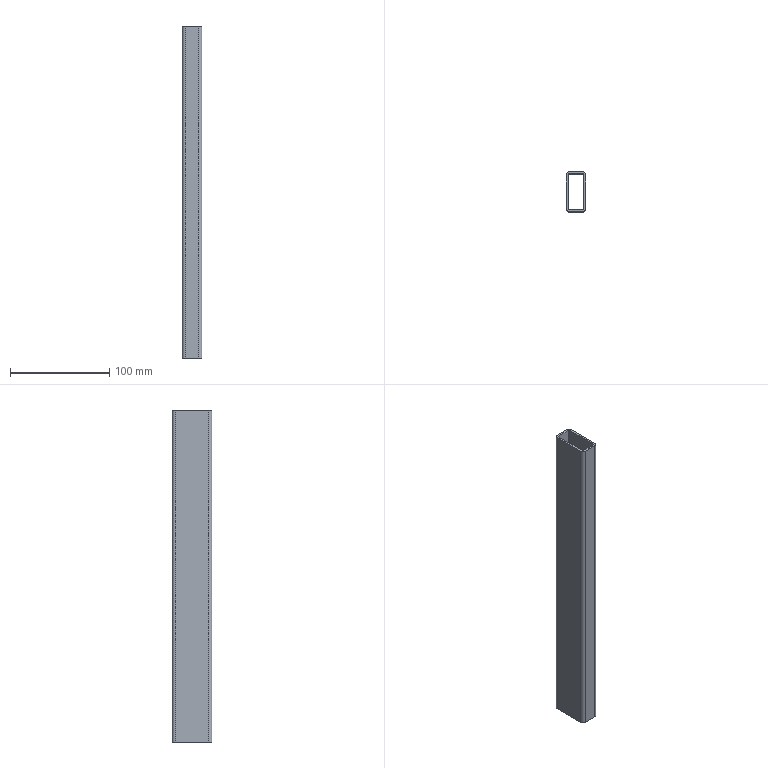Part | STEP file | CSN EN 10305-5 - 40 x 20 x 2  - 330 | 1 solid | 18 faces | box 20 x 40 x 335 mm | volume 72739 mm3 | plane 10 | cylinder 8 | commonest cylinder face diameters 2 x4 6 x4
STEP:
#1=CARTESIAN_POINT('',(0.,0.,0.));
#2=DIRECTION('',(0.,0.,1.));
#3=DIRECTION('',(1.,0.,0.));
#4=AXIS2_PLACEMENT_3D('',#1,#2,#3);
#5=CARTESIAN_POINT('',(-7.,-18.,335.));
#6=VERTEX_POINT('',#5);
#7=CARTESIAN_POINT('',(7.,-18.,335.));
#8=VERTEX_POINT('',#7);
#9=CARTESIAN_POINT('',(3.5,-18.,335.));
#10=DIRECTION('',(1.,0.,0.));
#11=VECTOR('',#10,1.);
#12=LINE('',#9,#11);
#13=CARTESIAN_POINT('',(7.,-18.,0.));
#14=DIRECTION('',(0.,-1.,0.));
#15=DIRECTION('',(0.,0.,-1.));
#16=AXIS2_PLACEMENT_3D('',#13,#14,#15);
#17=PLANE('',#16);
#18=CARTESIAN_POINT('',(-335.,-3.5));
#19=DIRECTION('',(0.,1.));
#20=VECTOR('',#19,1.);
#21=LINE('',#18,#20);
#22=(GEOMETRIC_REPRESENTATION_CONTEXT(2)PARAMETRIC_REPRESENTATION_CONTEXT()REPRESENTATION_CONTEXT('',''));
#23=DEFINITIONAL_REPRESENTATION('',(#21),#22);
#24=PCURVE('',#17,#23);
#25=CARTESIAN_POINT('',(0.,0.,335.));
#26=DIRECTION('',(0.,0.,1.));
#27=DIRECTION('',(1.,0.,0.));
#28=AXIS2_PLACEMENT_3D('',#25,#26,#27);
#29=PLANE('',#28);
#30=CARTESIAN_POINT('',(3.5,-18.));
#31=DIRECTION('',(1.,0.));
#32=VECTOR('',#31,1.);
#33=LINE('',#30,#32);
#34=(GEOMETRIC_REPRESENTATION_CONTEXT(2)PARAMETRIC_REPRESENTATION_CONTEXT()REPRESENTATION_CONTEXT('',''));
#35=DEFINITIONAL_REPRESENTATION('',(#33),#34);
#36=PCURVE('',#29,#35);
#37=SURFACE_CURVE('',#12,(#24,#36),.PCURVE_S1.);
#38=EDGE_CURVE('',#6,#8,#37,.T.);
#39=ORIENTED_EDGE('',*,*,#38,.T.);
#40=CARTESIAN_POINT('',(7.,-18.,0.));
#41=VERTEX_POINT('',#40);
#42=CARTESIAN_POINT('',(7.,-18.,0.));
#43=DIRECTION('',(0.,0.,1.));
#44=VECTOR('',#43,1.);
#45=LINE('',#42,#44);
#46=CARTESIAN_POINT('',(0.,0.));
#47=DIRECTION('',(-1.,0.));
#48=VECTOR('',#47,1.);
#49=LINE('',#46,#48);
#50=(GEOMETRIC_REPRESENTATION_CONTEXT(2)PARAMETRIC_REPRESENTATION_CONTEXT()REPRESENTATION_CONTEXT('',''));
#51=DEFINITIONAL_REPRESENTATION('',(#49),#50);
#52=PCURVE('',#17,#51);
#53=CARTESIAN_POINT('',(7.,-17.,0.));
#54=DIRECTION('',(0.,0.,1.));
#55=DIRECTION('',(0.,1.,0.));
#56=AXIS2_PLACEMENT_3D('',#53,#54,#55);
#57=CYLINDRICAL_SURFACE('',#56,1.);
#58=CARTESIAN_POINT('',(3.142,0.));
#59=DIRECTION('',(0.,1.));
#60=VECTOR('',#59,1.);
#61=LINE('',#58,#60);
#62=(GEOMETRIC_REPRESENTATION_CONTEXT(2)PARAMETRIC_REPRESENTATION_CONTEXT()REPRESENTATION_CONTEXT('',''));
#63=DEFINITIONAL_REPRESENTATION('',(#61),#62);
#64=PCURVE('',#57,#63);
#65=SURFACE_CURVE('',#45,(#52,#64),.PCURVE_S1.);
#66=EDGE_CURVE('',#41,#8,#65,.T.);
#67=ORIENTED_EDGE('',*,*,#66,.F.);
#68=CARTESIAN_POINT('',(-7.,-18.,0.));
#69=VERTEX_POINT('',#68);
#70=CARTESIAN_POINT('',(3.5,-18.,0.));
#71=DIRECTION('',(1.,0.,0.));
#72=VECTOR('',#71,1.);
#73=LINE('',#70,#72);
#74=CARTESIAN_POINT('',(0.,-3.5));
#75=DIRECTION('',(0.,1.));
#76=VECTOR('',#75,1.);
#77=LINE('',#74,#76);
#78=(GEOMETRIC_REPRESENTATION_CONTEXT(2)PARAMETRIC_REPRESENTATION_CONTEXT()REPRESENTATION_CONTEXT('',''));
#79=DEFINITIONAL_REPRESENTATION('',(#77),#78);
#80=PCURVE('',#17,#79);
#81=CARTESIAN_POINT('',(0.,0.,0.));
#82=DIRECTION('',(0.,0.,1.));
#83=DIRECTION('',(1.,0.,0.));
#84=AXIS2_PLACEMENT_3D('',#81,#82,#83);
#85=PLANE('',#84);
#86=CARTESIAN_POINT('',(3.5,-18.));
#87=DIRECTION('',(1.,0.));
#88=VECTOR('',#87,1.);
#89=LINE('',#86,#88);
#90=(GEOMETRIC_REPRESENTATION_CONTEXT(2)PARAMETRIC_REPRESENTATION_CONTEXT()REPRESENTATION_CONTEXT('',''));
#91=DEFINITIONAL_REPRESENTATION('',(#89),#90);
#92=PCURVE('',#85,#91);
#93=SURFACE_CURVE('',#73,(#80,#92),.PCURVE_S1.);
#94=EDGE_CURVE('',#69,#41,#93,.T.);
#95=ORIENTED_EDGE('',*,*,#94,.F.);
#96=CARTESIAN_POINT('',(-7.,-18.,0.));
#97=DIRECTION('',(0.,0.,1.));
#98=VECTOR('',#97,1.);
#99=LINE('',#96,#98);
#100=CARTESIAN_POINT('',(0.,-14.));
#101=DIRECTION('',(-1.,0.));
#102=VECTOR('',#101,1.);
#103=LINE('',#100,#102);
#104=(GEOMETRIC_REPRESENTATION_CONTEXT(2)PARAMETRIC_REPRESENTATION_CONTEXT()REPRESENTATION_CONTEXT('',''));
#105=DEFINITIONAL_REPRESENTATION('',(#103),#104);
#106=PCURVE('',#17,#105);
#107=CARTESIAN_POINT('',(-7.,-17.,0.));
#108=DIRECTION('',(0.,0.,1.));
#109=DIRECTION('',(1.,0.,0.));
#110=AXIS2_PLACEMENT_3D('',#107,#108,#109);
#111=CYLINDRICAL_SURFACE('',#110,1.);
#112=CARTESIAN_POINT('',(4.712,0.));
#113=DIRECTION('',(0.,1.));
#114=VECTOR('',#113,1.);
#115=LINE('',#112,#114);
#116=(GEOMETRIC_REPRESENTATION_CONTEXT(2)PARAMETRIC_REPRESENTATION_CONTEXT()REPRESENTATION_CONTEXT('',''));
#117=DEFINITIONAL_REPRESENTATION('',(#115),#116);
#118=PCURVE('',#111,#117);
#119=SURFACE_CURVE('',#99,(#106,#118),.PCURVE_S1.);
#120=EDGE_CURVE('',#69,#6,#119,.T.);
#121=ORIENTED_EDGE('',*,*,#120,.T.);
#122=EDGE_LOOP('',(#39,#67,#95,#121));
#123=FACE_BOUND('',#122,.T.);
#124=ADVANCED_FACE('',(#123),#17,.F.);
#125=ORIENTED_EDGE('',*,*,#66,.F.);
#126=CARTESIAN_POINT('',(8.,-17.,0.));
#127=VERTEX_POINT('',#126);
#128=CARTESIAN_POINT('',(7.,-17.,0.));
#129=DIRECTION('',(0.,0.,1.));
#130=DIRECTION('',(0.,1.,0.));
#131=AXIS2_PLACEMENT_3D('',#128,#129,#130);
#132=CIRCLE('',#131,1.);
#133=CARTESIAN_POINT('',(0.,0.));
#134=DIRECTION('',(1.,0.));
#135=VECTOR('',#134,1.);
#136=LINE('',#133,#135);
#137=(GEOMETRIC_REPRESENTATION_CONTEXT(2)PARAMETRIC_REPRESENTATION_CONTEXT()REPRESENTATION_CONTEXT('',''));
#138=DEFINITIONAL_REPRESENTATION('',(#136),#137);
#139=PCURVE('',#57,#138);
#140=CARTESIAN_POINT('',(7.,-17.));
#141=DIRECTION('',(0.,1.));
#142=AXIS2_PLACEMENT_2D('',#140,#141);
#143=CIRCLE('',#142,1.);
#144=(GEOMETRIC_REPRESENTATION_CONTEXT(2)PARAMETRIC_REPRESENTATION_CONTEXT()REPRESENTATION_CONTEXT('',''));
#145=DEFINITIONAL_REPRESENTATION('',(#143),#144);
#146=PCURVE('',#85,#145);
#147=SURFACE_CURVE('',#132,(#139,#146),.PCURVE_S1.);
#148=EDGE_CURVE('',#41,#127,#147,.T.);
#149=ORIENTED_EDGE('',*,*,#148,.T.);
#150=CARTESIAN_POINT('',(8.,-17.,335.));
#151=VERTEX_POINT('',#150);
#152=CARTESIAN_POINT('',(8.,-17.,0.));
#153=DIRECTION('',(0.,0.,1.));
#154=VECTOR('',#153,1.);
#155=LINE('',#152,#154);
#156=CARTESIAN_POINT('',(4.712,0.));
#157=DIRECTION('',(0.,1.));
#158=VECTOR('',#157,1.);
#159=LINE('',#156,#158);
#160=(GEOMETRIC_REPRESENTATION_CONTEXT(2)PARAMETRIC_REPRESENTATION_CONTEXT()REPRESENTATION_CONTEXT('',''));
#161=DEFINITIONAL_REPRESENTATION('',(#159),#160);
#162=PCURVE('',#57,#161);
#163=CARTESIAN_POINT('',(8.,17.,0.));
#164=DIRECTION('',(1.,0.,0.));
#165=DIRECTION('',(0.,0.,-1.));
#166=AXIS2_PLACEMENT_3D('',#163,#164,#165);
#167=PLANE('',#166);
#168=CARTESIAN_POINT('',(0.,-34.));
#169=DIRECTION('',(-1.,0.));
#170=VECTOR('',#169,1.);
#171=LINE('',#168,#170);
#172=(GEOMETRIC_REPRESENTATION_CONTEXT(2)PARAMETRIC_REPRESENTATION_CONTEXT()REPRESENTATION_CONTEXT('',''));
#173=DEFINITIONAL_REPRESENTATION('',(#171),#172);
#174=PCURVE('',#167,#173);
#175=SURFACE_CURVE('',#155,(#162,#174),.PCURVE_S1.);
#176=EDGE_CURVE('',#127,#151,#175,.T.);
#177=ORIENTED_EDGE('',*,*,#176,.T.);
#178=CARTESIAN_POINT('',(7.,-17.,335.));
#179=DIRECTION('',(0.,0.,1.));
#180=DIRECTION('',(0.,1.,0.));
#181=AXIS2_PLACEMENT_3D('',#178,#179,#180);
#182=CIRCLE('',#181,1.);
#183=CARTESIAN_POINT('',(0.,335.));
#184=DIRECTION('',(1.,0.));
#185=VECTOR('',#184,1.);
#186=LINE('',#183,#185);
#187=(GEOMETRIC_REPRESENTATION_CONTEXT(2)PARAMETRIC_REPRESENTATION_CONTEXT()REPRESENTATION_CONTEXT('',''));
#188=DEFINITIONAL_REPRESENTATION('',(#186),#187);
#189=PCURVE('',#57,#188);
#190=CARTESIAN_POINT('',(7.,-17.));
#191=DIRECTION('',(0.,1.));
#192=AXIS2_PLACEMENT_2D('',#190,#191);
#193=CIRCLE('',#192,1.);
#194=(GEOMETRIC_REPRESENTATION_CONTEXT(2)PARAMETRIC_REPRESENTATION_CONTEXT()REPRESENTATION_CONTEXT('',''));
#195=DEFINITIONAL_REPRESENTATION('',(#193),#194);
#196=PCURVE('',#29,#195);
#197=SURFACE_CURVE('',#182,(#189,#196),.PCURVE_S1.);
#198=EDGE_CURVE('',#8,#151,#197,.T.);
#199=ORIENTED_EDGE('',*,*,#198,.F.);
#200=EDGE_LOOP('',(#125,#149,#177,#199));
#201=FACE_BOUND('',#200,.F.);
#202=ADVANCED_FACE('',(#201),#57,.F.);
#203=CARTESIAN_POINT('',(8.,17.,335.));
#204=VERTEX_POINT('',#203);
#205=CARTESIAN_POINT('',(8.,8.5,335.));
#206=DIRECTION('',(0.,1.,0.));
#207=VECTOR('',#206,1.);
#208=LINE('',#205,#207);
#209=CARTESIAN_POINT('',(-335.,-8.5));
#210=DIRECTION('',(0.,1.));
#211=VECTOR('',#210,1.);
#212=LINE('',#209,#211);
#213=(GEOMETRIC_REPRESENTATION_CONTEXT(2)PARAMETRIC_REPRESENTATION_CONTEXT()REPRESENTATION_CONTEXT('',''));
#214=DEFINITIONAL_REPRESENTATION('',(#212),#213);
#215=PCURVE('',#167,#214);
#216=CARTESIAN_POINT('',(8.,8.5));
#217=DIRECTION('',(0.,1.));
#218=VECTOR('',#217,1.);
#219=LINE('',#216,#218);
#220=(GEOMETRIC_REPRESENTATION_CONTEXT(2)PARAMETRIC_REPRESENTATION_CONTEXT()REPRESENTATION_CONTEXT('',''));
#221=DEFINITIONAL_REPRESENTATION('',(#219),#220);
#222=PCURVE('',#29,#221);
#223=SURFACE_CURVE('',#208,(#215,#222),.PCURVE_S1.);
#224=EDGE_CURVE('',#151,#204,#223,.T.);
#225=ORIENTED_EDGE('',*,*,#224,.T.);
#226=CARTESIAN_POINT('',(8.,17.,0.));
#227=VERTEX_POINT('',#226);
#228=CARTESIAN_POINT('',(8.,17.,0.));
#229=DIRECTION('',(0.,0.,1.));
#230=VECTOR('',#229,1.);
#231=LINE('',#228,#230);
#232=CARTESIAN_POINT('',(0.,0.));
#233=DIRECTION('',(-1.,0.));
#234=VECTOR('',#233,1.);
#235=LINE('',#232,#234);
#236=(GEOMETRIC_REPRESENTATION_CONTEXT(2)PARAMETRIC_REPRESENTATION_CONTEXT()REPRESENTATION_CONTEXT('',''));
#237=DEFINITIONAL_REPRESENTATION('',(#235),#236);
#238=PCURVE('',#167,#237);
#239=CARTESIAN_POINT('',(7.,17.,0.));
#240=DIRECTION('',(0.,0.,1.));
#241=DIRECTION('',(-1.,0.,0.));
#242=AXIS2_PLACEMENT_3D('',#239,#240,#241);
#243=CYLINDRICAL_SURFACE('',#242,1.);
#244=CARTESIAN_POINT('',(3.142,0.));
#245=DIRECTION('',(0.,1.));
#246=VECTOR('',#245,1.);
#247=LINE('',#244,#246);
#248=(GEOMETRIC_REPRESENTATION_CONTEXT(2)PARAMETRIC_REPRESENTATION_CONTEXT()REPRESENTATION_CONTEXT('',''));
#249=DEFINITIONAL_REPRESENTATION('',(#247),#248);
#250=PCURVE('',#243,#249);
#251=SURFACE_CURVE('',#231,(#238,#250),.PCURVE_S1.);
#252=EDGE_CURVE('',#227,#204,#251,.T.);
#253=ORIENTED_EDGE('',*,*,#252,.F.);
#254=CARTESIAN_POINT('',(8.,8.5,0.));
#255=DIRECTION('',(0.,1.,0.));
#256=VECTOR('',#255,1.);
#257=LINE('',#254,#256);
#258=CARTESIAN_POINT('',(0.,-8.5));
#259=DIRECTION('',(0.,1.));
#260=VECTOR('',#259,1.);
#261=LINE('',#258,#260);
#262=(GEOMETRIC_REPRESENTATION_CONTEXT(2)PARAMETRIC_REPRESENTATION_CONTEXT()REPRESENTATION_CONTEXT('',''));
#263=DEFINITIONAL_REPRESENTATION('',(#261),#262);
#264=PCURVE('',#167,#263);
#265=CARTESIAN_POINT('',(8.,8.5));
#266=DIRECTION('',(0.,1.));
#267=VECTOR('',#266,1.);
#268=LINE('',#265,#267);
#269=(GEOMETRIC_REPRESENTATION_CONTEXT(2)PARAMETRIC_REPRESENTATION_CONTEXT()REPRESENTATION_CONTEXT('',''));
#270=DEFINITIONAL_REPRESENTATION('',(#268),#269);
#271=PCURVE('',#85,#270);
#272=SURFACE_CURVE('',#257,(#264,#271),.PCURVE_S1.);
#273=EDGE_CURVE('',#127,#227,#272,.T.);
#274=ORIENTED_EDGE('',*,*,#273,.F.);
#275=ORIENTED_EDGE('',*,*,#176,.T.);
#276=EDGE_LOOP('',(#225,#253,#274,#275));
#277=FACE_BOUND('',#276,.T.);
#278=ADVANCED_FACE('',(#277),#167,.F.);
#279=ORIENTED_EDGE('',*,*,#252,.F.);
#280=CARTESIAN_POINT('',(7.,18.,0.));
#281=VERTEX_POINT('',#280);
#282=CARTESIAN_POINT('',(7.,17.,0.));
#283=DIRECTION('',(0.,0.,1.));
#284=DIRECTION('',(-1.,0.,0.));
#285=AXIS2_PLACEMENT_3D('',#282,#283,#284);
#286=CIRCLE('',#285,1.);
#287=CARTESIAN_POINT('',(0.,0.));
#288=DIRECTION('',(1.,0.));
#289=VECTOR('',#288,1.);
#290=LINE('',#287,#289);
#291=(GEOMETRIC_REPRESENTATION_CONTEXT(2)PARAMETRIC_REPRESENTATION_CONTEXT()REPRESENTATION_CONTEXT('',''));
#292=DEFINITIONAL_REPRESENTATION('',(#290),#291);
#293=PCURVE('',#243,#292);
#294=CARTESIAN_POINT('',(7.,17.));
#295=DIRECTION('',(-1.,0.));
#296=AXIS2_PLACEMENT_2D('',#294,#295);
#297=CIRCLE('',#296,1.);
#298=(GEOMETRIC_REPRESENTATION_CONTEXT(2)PARAMETRIC_REPRESENTATION_CONTEXT()REPRESENTATION_CONTEXT('',''));
#299=DEFINITIONAL_REPRESENTATION('',(#297),#298);
#300=PCURVE('',#85,#299);
#301=SURFACE_CURVE('',#286,(#293,#300),.PCURVE_S1.);
#302=EDGE_CURVE('',#227,#281,#301,.T.);
#303=ORIENTED_EDGE('',*,*,#302,.T.);
#304=CARTESIAN_POINT('',(7.,18.,335.));
#305=VERTEX_POINT('',#304);
#306=CARTESIAN_POINT('',(7.,18.,0.));
#307=DIRECTION('',(0.,0.,1.));
#308=VECTOR('',#307,1.);
#309=LINE('',#306,#308);
#310=CARTESIAN_POINT('',(4.712,0.));
#311=DIRECTION('',(0.,1.));
#312=VECTOR('',#311,1.);
#313=LINE('',#310,#312);
#314=(GEOMETRIC_REPRESENTATION_CONTEXT(2)PARAMETRIC_REPRESENTATION_CONTEXT()REPRESENTATION_CONTEXT('',''));
#315=DEFINITIONAL_REPRESENTATION('',(#313),#314);
#316=PCURVE('',#243,#315);
#317=CARTESIAN_POINT('',(-7.,18.,0.));
#318=DIRECTION('',(0.,1.,0.));
#319=DIRECTION('',(0.,0.,1.));
#320=AXIS2_PLACEMENT_3D('',#317,#318,#319);
#321=PLANE('',#320);
#322=CARTESIAN_POINT('',(0.,14.));
#323=DIRECTION('',(1.,0.));
#324=VECTOR('',#323,1.);
#325=LINE('',#322,#324);
#326=(GEOMETRIC_REPRESENTATION_CONTEXT(2)PARAMETRIC_REPRESENTATION_CONTEXT()REPRESENTATION_CONTEXT('',''));
#327=DEFINITIONAL_REPRESENTATION('',(#325),#326);
#328=PCURVE('',#321,#327);
#329=SURFACE_CURVE('',#309,(#316,#328),.PCURVE_S1.);
#330=EDGE_CURVE('',#281,#305,#329,.T.);
#331=ORIENTED_EDGE('',*,*,#330,.T.);
#332=CARTESIAN_POINT('',(7.,17.,335.));
#333=DIRECTION('',(0.,0.,1.));
#334=DIRECTION('',(-1.,0.,0.));
#335=AXIS2_PLACEMENT_3D('',#332,#333,#334);
#336=CIRCLE('',#335,1.);
#337=CARTESIAN_POINT('',(0.,335.));
#338=DIRECTION('',(1.,0.));
#339=VECTOR('',#338,1.);
#340=LINE('',#337,#339);
#341=(GEOMETRIC_REPRESENTATION_CONTEXT(2)PARAMETRIC_REPRESENTATION_CONTEXT()REPRESENTATION_CONTEXT('',''));
#342=DEFINITIONAL_REPRESENTATION('',(#340),#341);
#343=PCURVE('',#243,#342);
#344=CARTESIAN_POINT('',(7.,17.));
#345=DIRECTION('',(-1.,0.));
#346=AXIS2_PLACEMENT_2D('',#344,#345);
#347=CIRCLE('',#346,1.);
#348=(GEOMETRIC_REPRESENTATION_CONTEXT(2)PARAMETRIC_REPRESENTATION_CONTEXT()REPRESENTATION_CONTEXT('',''));
#349=DEFINITIONAL_REPRESENTATION('',(#347),#348);
#350=PCURVE('',#29,#349);
#351=SURFACE_CURVE('',#336,(#343,#350),.PCURVE_S1.);
#352=EDGE_CURVE('',#204,#305,#351,.T.);
#353=ORIENTED_EDGE('',*,*,#352,.F.);
#354=EDGE_LOOP('',(#279,#303,#331,#353));
#355=FACE_BOUND('',#354,.F.);
#356=ADVANCED_FACE('',(#355),#243,.F.);
#357=CARTESIAN_POINT('',(10.,17.,335.));
#358=VERTEX_POINT('',#357);
#359=CARTESIAN_POINT('',(10.,-17.,335.));
#360=VERTEX_POINT('',#359);
#361=CARTESIAN_POINT('',(10.,8.5,335.));
#362=DIRECTION('',(0.,-1.,0.));
#363=VECTOR('',#362,1.);
#364=LINE('',#361,#363);
#365=CARTESIAN_POINT('',(10.,17.,0.));
#366=DIRECTION('',(1.,0.,0.));
#367=DIRECTION('',(0.,0.,-1.));
#368=AXIS2_PLACEMENT_3D('',#365,#366,#367);
#369=PLANE('',#368);
#370=CARTESIAN_POINT('',(-335.,-8.5));
#371=DIRECTION('',(0.,-1.));
#372=VECTOR('',#371,1.);
#373=LINE('',#370,#372);
#374=(GEOMETRIC_REPRESENTATION_CONTEXT(2)PARAMETRIC_REPRESENTATION_CONTEXT()REPRESENTATION_CONTEXT('',''));
#375=DEFINITIONAL_REPRESENTATION('',(#373),#374);
#376=PCURVE('',#369,#375);
#377=CARTESIAN_POINT('',(10.,8.5));
#378=DIRECTION('',(0.,-1.));
#379=VECTOR('',#378,1.);
#380=LINE('',#377,#379);
#381=(GEOMETRIC_REPRESENTATION_CONTEXT(2)PARAMETRIC_REPRESENTATION_CONTEXT()REPRESENTATION_CONTEXT('',''));
#382=DEFINITIONAL_REPRESENTATION('',(#380),#381);
#383=PCURVE('',#29,#382);
#384=SURFACE_CURVE('',#364,(#376,#383),.PCURVE_S1.);
#385=EDGE_CURVE('',#358,#360,#384,.T.);
#386=ORIENTED_EDGE('',*,*,#385,.T.);
#387=CARTESIAN_POINT('',(10.,-17.,0.));
#388=VERTEX_POINT('',#387);
#389=CARTESIAN_POINT('',(10.,-17.,0.));
#390=DIRECTION('',(0.,0.,1.));
#391=VECTOR('',#390,1.);
#392=LINE('',#389,#391);
#393=CARTESIAN_POINT('',(0.,-34.));
#394=DIRECTION('',(-1.,0.));
#395=VECTOR('',#394,1.);
#396=LINE('',#393,#395);
#397=(GEOMETRIC_REPRESENTATION_CONTEXT(2)PARAMETRIC_REPRESENTATION_CONTEXT()REPRESENTATION_CONTEXT('',''));
#398=DEFINITIONAL_REPRESENTATION('',(#396),#397);
#399=PCURVE('',#369,#398);
#400=CARTESIAN_POINT('',(7.,-17.,0.));
#401=DIRECTION('',(0.,0.,1.));
#402=DIRECTION('',(0.,1.,0.));
#403=AXIS2_PLACEMENT_3D('',#400,#401,#402);
#404=CYLINDRICAL_SURFACE('',#403,3.);
#405=CARTESIAN_POINT('',(4.712,0.));
#406=DIRECTION('',(0.,1.));
#407=VECTOR('',#406,1.);
#408=LINE('',#405,#407);
#409=(GEOMETRIC_REPRESENTATION_CONTEXT(2)PARAMETRIC_REPRESENTATION_CONTEXT()REPRESENTATION_CONTEXT('',''));
#410=DEFINITIONAL_REPRESENTATION('',(#408),#409);
#411=PCURVE('',#404,#410);
#412=SURFACE_CURVE('',#392,(#399,#411),.PCURVE_S1.);
#413=EDGE_CURVE('',#388,#360,#412,.T.);
#414=ORIENTED_EDGE('',*,*,#413,.F.);
#415=CARTESIAN_POINT('',(10.,17.,0.));
#416=VERTEX_POINT('',#415);
#417=CARTESIAN_POINT('',(10.,8.5,0.));
#418=DIRECTION('',(0.,-1.,0.));
#419=VECTOR('',#418,1.);
#420=LINE('',#417,#419);
#421=CARTESIAN_POINT('',(0.,-8.5));
#422=DIRECTION('',(0.,-1.));
#423=VECTOR('',#422,1.);
#424=LINE('',#421,#423);
#425=(GEOMETRIC_REPRESENTATION_CONTEXT(2)PARAMETRIC_REPRESENTATION_CONTEXT()REPRESENTATION_CONTEXT('',''));
#426=DEFINITIONAL_REPRESENTATION('',(#424),#425);
#427=PCURVE('',#369,#426);
#428=CARTESIAN_POINT('',(10.,8.5));
#429=DIRECTION('',(0.,-1.));
#430=VECTOR('',#429,1.);
#431=LINE('',#428,#430);
#432=(GEOMETRIC_REPRESENTATION_CONTEXT(2)PARAMETRIC_REPRESENTATION_CONTEXT()REPRESENTATION_CONTEXT('',''));
#433=DEFINITIONAL_REPRESENTATION('',(#431),#432);
#434=PCURVE('',#85,#433);
#435=SURFACE_CURVE('',#420,(#427,#434),.PCURVE_S1.);
#436=EDGE_CURVE('',#416,#388,#435,.T.);
#437=ORIENTED_EDGE('',*,*,#436,.F.);
#438=CARTESIAN_POINT('',(10.,17.,0.));
#439=DIRECTION('',(0.,0.,1.));
#440=VECTOR('',#439,1.);
#441=LINE('',#438,#440);
#442=CARTESIAN_POINT('',(0.,0.));
#443=DIRECTION('',(-1.,0.));
#444=VECTOR('',#443,1.);
#445=LINE('',#442,#444);
#446=(GEOMETRIC_REPRESENTATION_CONTEXT(2)PARAMETRIC_REPRESENTATION_CONTEXT()REPRESENTATION_CONTEXT('',''));
#447=DEFINITIONAL_REPRESENTATION('',(#445),#446);
#448=PCURVE('',#369,#447);
#449=CARTESIAN_POINT('',(7.,17.,0.));
#450=DIRECTION('',(0.,0.,1.));
#451=DIRECTION('',(-1.,0.,0.));
#452=AXIS2_PLACEMENT_3D('',#449,#450,#451);
#453=CYLINDRICAL_SURFACE('',#452,3.);
#454=CARTESIAN_POINT('',(3.142,0.));
#455=DIRECTION('',(0.,1.));
#456=VECTOR('',#455,1.);
#457=LINE('',#454,#456);
#458=(GEOMETRIC_REPRESENTATION_CONTEXT(2)PARAMETRIC_REPRESENTATION_CONTEXT()REPRESENTATION_CONTEXT('',''));
#459=DEFINITIONAL_REPRESENTATION('',(#457),#458);
#460=PCURVE('',#453,#459);
#461=SURFACE_CURVE('',#441,(#448,#460),.PCURVE_S1.);
#462=EDGE_CURVE('',#416,#358,#461,.T.);
#463=ORIENTED_EDGE('',*,*,#462,.T.);
#464=EDGE_LOOP('',(#386,#414,#437,#463));
#465=FACE_BOUND('',#464,.T.);
#466=ADVANCED_FACE('',(#465),#369,.T.);
#467=CARTESIAN_POINT('',(7.,-20.,335.));
#468=VERTEX_POINT('',#467);
#469=CARTESIAN_POINT('',(7.,-17.,335.));
#470=DIRECTION('',(0.,0.,-1.));
#471=DIRECTION('',(0.,1.,0.));
#472=AXIS2_PLACEMENT_3D('',#469,#470,#471);
#473=CIRCLE('',#472,3.);
#474=CARTESIAN_POINT('',(6.283,335.));
#475=DIRECTION('',(-1.,0.));
#476=VECTOR('',#475,1.);
#477=LINE('',#474,#476);
#478=(GEOMETRIC_REPRESENTATION_CONTEXT(2)PARAMETRIC_REPRESENTATION_CONTEXT()REPRESENTATION_CONTEXT('',''));
#479=DEFINITIONAL_REPRESENTATION('',(#477),#478);
#480=PCURVE('',#404,#479);
#481=CARTESIAN_POINT('',(7.,-14.));
#482=CARTESIAN_POINT('',(12.196,-14.));
#483=CARTESIAN_POINT('',(9.598,-18.5));
#484=CARTESIAN_POINT('',(7.,-23.));
#485=CARTESIAN_POINT('',(4.402,-18.5));
#486=CARTESIAN_POINT('',(1.804,-14.));
#487=CARTESIAN_POINT('',(7.,-14.));
#488=(BOUNDED_CURVE()B_SPLINE_CURVE(2,(#481,#482,#483,#484,#485,#486,#487),.UNSPECIFIED.,.T.,.F.)B_SPLINE_CURVE_WITH_KNOTS((1,2,2,2,2,1),(-2.094,0.,2.094,4.189,6.283,8.378),.UNSPECIFIED.)CURVE()GEOMETRIC_REPRESENTATION_ITEM()RATIONAL_B_SPLINE_CURVE((1.,0.5,1.,0.5,1.,0.5,1.))REPRESENTATION_ITEM(''));
#489=(GEOMETRIC_REPRESENTATION_CONTEXT(2)PARAMETRIC_REPRESENTATION_CONTEXT()REPRESENTATION_CONTEXT('',''));
#490=DEFINITIONAL_REPRESENTATION('',(#488),#489);
#491=PCURVE('',#29,#490);
#492=SURFACE_CURVE('',#473,(#480,#491),.PCURVE_S1.);
#493=EDGE_CURVE('',#360,#468,#492,.T.);
#494=ORIENTED_EDGE('',*,*,#493,.T.);
#495=CARTESIAN_POINT('',(7.,-20.,0.));
#496=VERTEX_POINT('',#495);
#497=CARTESIAN_POINT('',(7.,-20.,0.));
#498=DIRECTION('',(0.,0.,1.));
#499=VECTOR('',#498,1.);
#500=LINE('',#497,#499);
#501=CARTESIAN_POINT('',(3.142,0.));
#502=DIRECTION('',(0.,1.));
#503=VECTOR('',#502,1.);
#504=LINE('',#501,#503);
#505=(GEOMETRIC_REPRESENTATION_CONTEXT(2)PARAMETRIC_REPRESENTATION_CONTEXT()REPRESENTATION_CONTEXT('',''));
#506=DEFINITIONAL_REPRESENTATION('',(#504),#505);
#507=PCURVE('',#404,#506);
#508=CARTESIAN_POINT('',(7.,-20.,0.));
#509=DIRECTION('',(0.,-1.,0.));
#510=DIRECTION('',(0.,0.,-1.));
#511=AXIS2_PLACEMENT_3D('',#508,#509,#510);
#512=PLANE('',#511);
#513=CARTESIAN_POINT('',(0.,0.));
#514=DIRECTION('',(-1.,0.));
#515=VECTOR('',#514,1.);
#516=LINE('',#513,#515);
#517=(GEOMETRIC_REPRESENTATION_CONTEXT(2)PARAMETRIC_REPRESENTATION_CONTEXT()REPRESENTATION_CONTEXT('',''));
#518=DEFINITIONAL_REPRESENTATION('',(#516),#517);
#519=PCURVE('',#512,#518);
#520=SURFACE_CURVE('',#500,(#507,#519),.PCURVE_S1.);
#521=EDGE_CURVE('',#496,#468,#520,.T.);
#522=ORIENTED_EDGE('',*,*,#521,.F.);
#523=CARTESIAN_POINT('',(7.,-17.,0.));
#524=DIRECTION('',(0.,0.,-1.));
#525=DIRECTION('',(0.,1.,0.));
#526=AXIS2_PLACEMENT_3D('',#523,#524,#525);
#527=CIRCLE('',#526,3.);
#528=CARTESIAN_POINT('',(6.283,0.));
#529=DIRECTION('',(-1.,0.));
#530=VECTOR('',#529,1.);
#531=LINE('',#528,#530);
#532=(GEOMETRIC_REPRESENTATION_CONTEXT(2)PARAMETRIC_REPRESENTATION_CONTEXT()REPRESENTATION_CONTEXT('',''));
#533=DEFINITIONAL_REPRESENTATION('',(#531),#532);
#534=PCURVE('',#404,#533);
#535=CARTESIAN_POINT('',(7.,-14.));
#536=CARTESIAN_POINT('',(12.196,-14.));
#537=CARTESIAN_POINT('',(9.598,-18.5));
#538=CARTESIAN_POINT('',(7.,-23.));
#539=CARTESIAN_POINT('',(4.402,-18.5));
#540=CARTESIAN_POINT('',(1.804,-14.));
#541=CARTESIAN_POINT('',(7.,-14.));
#542=(BOUNDED_CURVE()B_SPLINE_CURVE(2,(#535,#536,#537,#538,#539,#540,#541),.UNSPECIFIED.,.T.,.F.)B_SPLINE_CURVE_WITH_KNOTS((1,2,2,2,2,1),(-2.094,0.,2.094,4.189,6.283,8.378),.UNSPECIFIED.)CURVE()GEOMETRIC_REPRESENTATION_ITEM()RATIONAL_B_SPLINE_CURVE((1.,0.5,1.,0.5,1.,0.5,1.))REPRESENTATION_ITEM(''));
#543=(GEOMETRIC_REPRESENTATION_CONTEXT(2)PARAMETRIC_REPRESENTATION_CONTEXT()REPRESENTATION_CONTEXT('',''));
#544=DEFINITIONAL_REPRESENTATION('',(#542),#543);
#545=PCURVE('',#85,#544);
#546=SURFACE_CURVE('',#527,(#534,#545),.PCURVE_S1.);
#547=EDGE_CURVE('',#388,#496,#546,.T.);
#548=ORIENTED_EDGE('',*,*,#547,.F.);
#549=ORIENTED_EDGE('',*,*,#413,.T.);
#550=EDGE_LOOP('',(#494,#522,#548,#549));
#551=FACE_BOUND('',#550,.T.);
#552=ADVANCED_FACE('',(#551),#404,.T.);
#553=CARTESIAN_POINT('',(-7.,-20.,335.));
#554=VERTEX_POINT('',#553);
#555=CARTESIAN_POINT('',(3.5,-20.,335.));
#556=DIRECTION('',(-1.,0.,0.));
#557=VECTOR('',#556,1.);
#558=LINE('',#555,#557);
#559=CARTESIAN_POINT('',(-335.,-3.5));
#560=DIRECTION('',(0.,-1.));
#561=VECTOR('',#560,1.);
#562=LINE('',#559,#561);
#563=(GEOMETRIC_REPRESENTATION_CONTEXT(2)PARAMETRIC_REPRESENTATION_CONTEXT()REPRESENTATION_CONTEXT('',''));
#564=DEFINITIONAL_REPRESENTATION('',(#562),#563);
#565=PCURVE('',#512,#564);
#566=CARTESIAN_POINT('',(3.5,-20.));
#567=DIRECTION('',(-1.,0.));
#568=VECTOR('',#567,1.);
#569=LINE('',#566,#568);
#570=(GEOMETRIC_REPRESENTATION_CONTEXT(2)PARAMETRIC_REPRESENTATION_CONTEXT()REPRESENTATION_CONTEXT('',''));
#571=DEFINITIONAL_REPRESENTATION('',(#569),#570);
#572=PCURVE('',#29,#571);
#573=SURFACE_CURVE('',#558,(#565,#572),.PCURVE_S1.);
#574=EDGE_CURVE('',#468,#554,#573,.T.);
#575=ORIENTED_EDGE('',*,*,#574,.T.);
#576=CARTESIAN_POINT('',(-7.,-20.,0.));
#577=VERTEX_POINT('',#576);
#578=CARTESIAN_POINT('',(-7.,-20.,0.));
#579=DIRECTION('',(0.,0.,1.));
#580=VECTOR('',#579,1.);
#581=LINE('',#578,#580);
#582=CARTESIAN_POINT('',(0.,-14.));
#583=DIRECTION('',(-1.,0.));
#584=VECTOR('',#583,1.);
#585=LINE('',#582,#584);
#586=(GEOMETRIC_REPRESENTATION_CONTEXT(2)PARAMETRIC_REPRESENTATION_CONTEXT()REPRESENTATION_CONTEXT('',''));
#587=DEFINITIONAL_REPRESENTATION('',(#585),#586);
#588=PCURVE('',#512,#587);
#589=CARTESIAN_POINT('',(-7.,-17.,0.));
#590=DIRECTION('',(0.,0.,1.));
#591=DIRECTION('',(1.,0.,0.));
#592=AXIS2_PLACEMENT_3D('',#589,#590,#591);
#593=CYLINDRICAL_SURFACE('',#592,3.);
#594=CARTESIAN_POINT('',(4.712,0.));
#595=DIRECTION('',(0.,1.));
#596=VECTOR('',#595,1.);
#597=LINE('',#594,#596);
#598=(GEOMETRIC_REPRESENTATION_CONTEXT(2)PARAMETRIC_REPRESENTATION_CONTEXT()REPRESENTATION_CONTEXT('',''));
#599=DEFINITIONAL_REPRESENTATION('',(#597),#598);
#600=PCURVE('',#593,#599);
#601=SURFACE_CURVE('',#581,(#588,#600),.PCURVE_S1.);
#602=EDGE_CURVE('',#577,#554,#601,.T.);
#603=ORIENTED_EDGE('',*,*,#602,.F.);
#604=CARTESIAN_POINT('',(3.5,-20.,0.));
#605=DIRECTION('',(-1.,0.,0.));
#606=VECTOR('',#605,1.);
#607=LINE('',#604,#606);
#608=CARTESIAN_POINT('',(0.,-3.5));
#609=DIRECTION('',(0.,-1.));
#610=VECTOR('',#609,1.);
#611=LINE('',#608,#610);
#612=(GEOMETRIC_REPRESENTATION_CONTEXT(2)PARAMETRIC_REPRESENTATION_CONTEXT()REPRESENTATION_CONTEXT('',''));
#613=DEFINITIONAL_REPRESENTATION('',(#611),#612);
#614=PCURVE('',#512,#613);
#615=CARTESIAN_POINT('',(3.5,-20.));
#616=DIRECTION('',(-1.,0.));
#617=VECTOR('',#616,1.);
#618=LINE('',#615,#617);
#619=(GEOMETRIC_REPRESENTATION_CONTEXT(2)PARAMETRIC_REPRESENTATION_CONTEXT()REPRESENTATION_CONTEXT('',''));
#620=DEFINITIONAL_REPRESENTATION('',(#618),#619);
#621=PCURVE('',#85,#620);
#622=SURFACE_CURVE('',#607,(#614,#621),.PCURVE_S1.);
#623=EDGE_CURVE('',#496,#577,#622,.T.);
#624=ORIENTED_EDGE('',*,*,#623,.F.);
#625=ORIENTED_EDGE('',*,*,#521,.T.);
#626=EDGE_LOOP('',(#575,#603,#624,#625));
#627=FACE_BOUND('',#626,.T.);
#628=ADVANCED_FACE('',(#627),#512,.T.);
#629=CARTESIAN_POINT('',(-10.,-17.,335.));
#630=VERTEX_POINT('',#629);
#631=CARTESIAN_POINT('',(-7.,-17.,335.));
#632=DIRECTION('',(0.,0.,-1.));
#633=DIRECTION('',(1.,0.,0.));
#634=AXIS2_PLACEMENT_3D('',#631,#632,#633);
#635=CIRCLE('',#634,3.);
#636=CARTESIAN_POINT('',(6.283,335.));
#637=DIRECTION('',(-1.,0.));
#638=VECTOR('',#637,1.);
#639=LINE('',#636,#638);
#640=(GEOMETRIC_REPRESENTATION_CONTEXT(2)PARAMETRIC_REPRESENTATION_CONTEXT()REPRESENTATION_CONTEXT('',''));
#641=DEFINITIONAL_REPRESENTATION('',(#639),#640);
#642=PCURVE('',#593,#641);
#643=CARTESIAN_POINT('',(-4.,-17.));
#644=CARTESIAN_POINT('',(-4.,-22.196));
#645=CARTESIAN_POINT('',(-8.5,-19.598));
#646=CARTESIAN_POINT('',(-13.,-17.));
#647=CARTESIAN_POINT('',(-8.5,-14.402));
#648=CARTESIAN_POINT('',(-4.,-11.804));
#649=CARTESIAN_POINT('',(-4.,-17.));
#650=(BOUNDED_CURVE()B_SPLINE_CURVE(2,(#643,#644,#645,#646,#647,#648,#649),.UNSPECIFIED.,.T.,.F.)B_SPLINE_CURVE_WITH_KNOTS((1,2,2,2,2,1),(-2.094,0.,2.094,4.189,6.283,8.378),.UNSPECIFIED.)CURVE()GEOMETRIC_REPRESENTATION_ITEM()RATIONAL_B_SPLINE_CURVE((1.,0.5,1.,0.5,1.,0.5,1.))REPRESENTATION_ITEM(''));
#651=(GEOMETRIC_REPRESENTATION_CONTEXT(2)PARAMETRIC_REPRESENTATION_CONTEXT()REPRESENTATION_CONTEXT('',''));
#652=DEFINITIONAL_REPRESENTATION('',(#650),#651);
#653=PCURVE('',#29,#652);
#654=SURFACE_CURVE('',#635,(#642,#653),.PCURVE_S1.);
#655=EDGE_CURVE('',#554,#630,#654,.T.);
#656=ORIENTED_EDGE('',*,*,#655,.T.);
#657=CARTESIAN_POINT('',(-10.,-17.,0.));
#658=VERTEX_POINT('',#657);
#659=CARTESIAN_POINT('',(-10.,-17.,0.));
#660=DIRECTION('',(0.,0.,1.));
#661=VECTOR('',#660,1.);
#662=LINE('',#659,#661);
#663=CARTESIAN_POINT('',(3.142,0.));
#664=DIRECTION('',(0.,1.));
#665=VECTOR('',#664,1.);
#666=LINE('',#663,#665);
#667=(GEOMETRIC_REPRESENTATION_CONTEXT(2)PARAMETRIC_REPRESENTATION_CONTEXT()REPRESENTATION_CONTEXT('',''));
#668=DEFINITIONAL_REPRESENTATION('',(#666),#667);
#669=PCURVE('',#593,#668);
#670=CARTESIAN_POINT('',(-10.,-17.,0.));
#671=DIRECTION('',(-1.,0.,0.));
#672=DIRECTION('',(0.,0.,1.));
#673=AXIS2_PLACEMENT_3D('',#670,#671,#672);
#674=PLANE('',#673);
#675=CARTESIAN_POINT('',(0.,0.));
#676=DIRECTION('',(1.,0.));
#677=VECTOR('',#676,1.);
#678=LINE('',#675,#677);
#679=(GEOMETRIC_REPRESENTATION_CONTEXT(2)PARAMETRIC_REPRESENTATION_CONTEXT()REPRESENTATION_CONTEXT('',''));
#680=DEFINITIONAL_REPRESENTATION('',(#678),#679);
#681=PCURVE('',#674,#680);
#682=SURFACE_CURVE('',#662,(#669,#681),.PCURVE_S1.);
#683=EDGE_CURVE('',#658,#630,#682,.T.);
#684=ORIENTED_EDGE('',*,*,#683,.F.);
#685=CARTESIAN_POINT('',(-7.,-17.,0.));
#686=DIRECTION('',(0.,0.,-1.));
#687=DIRECTION('',(1.,0.,0.));
#688=AXIS2_PLACEMENT_3D('',#685,#686,#687);
#689=CIRCLE('',#688,3.);
#690=CARTESIAN_POINT('',(6.283,0.));
#691=DIRECTION('',(-1.,0.));
#692=VECTOR('',#691,1.);
#693=LINE('',#690,#692);
#694=(GEOMETRIC_REPRESENTATION_CONTEXT(2)PARAMETRIC_REPRESENTATION_CONTEXT()REPRESENTATION_CONTEXT('',''));
#695=DEFINITIONAL_REPRESENTATION('',(#693),#694);
#696=PCURVE('',#593,#695);
#697=CARTESIAN_POINT('',(-4.,-17.));
#698=CARTESIAN_POINT('',(-4.,-22.196));
#699=CARTESIAN_POINT('',(-8.5,-19.598));
#700=CARTESIAN_POINT('',(-13.,-17.));
#701=CARTESIAN_POINT('',(-8.5,-14.402));
#702=CARTESIAN_POINT('',(-4.,-11.804));
#703=CARTESIAN_POINT('',(-4.,-17.));
#704=(BOUNDED_CURVE()B_SPLINE_CURVE(2,(#697,#698,#699,#700,#701,#702,#703),.UNSPECIFIED.,.T.,.F.)B_SPLINE_CURVE_WITH_KNOTS((1,2,2,2,2,1),(-2.094,0.,2.094,4.189,6.283,8.378),.UNSPECIFIED.)CURVE()GEOMETRIC_REPRESENTATION_ITEM()RATIONAL_B_SPLINE_CURVE((1.,0.5,1.,0.5,1.,0.5,1.))REPRESENTATION_ITEM(''));
#705=(GEOMETRIC_REPRESENTATION_CONTEXT(2)PARAMETRIC_REPRESENTATION_CONTEXT()REPRESENTATION_CONTEXT('',''));
#706=DEFINITIONAL_REPRESENTATION('',(#704),#705);
#707=PCURVE('',#85,#706);
#708=SURFACE_CURVE('',#689,(#696,#707),.PCURVE_S1.);
#709=EDGE_CURVE('',#577,#658,#708,.T.);
#710=ORIENTED_EDGE('',*,*,#709,.F.);
#711=ORIENTED_EDGE('',*,*,#602,.T.);
#712=EDGE_LOOP('',(#656,#684,#710,#711));
#713=FACE_BOUND('',#712,.T.);
#714=ADVANCED_FACE('',(#713),#593,.T.);
#715=CARTESIAN_POINT('',(-7.,18.,335.));
#716=VERTEX_POINT('',#715);
#717=CARTESIAN_POINT('',(-3.5,18.,335.));
#718=DIRECTION('',(-1.,0.,0.));
#719=VECTOR('',#718,1.);
#720=LINE('',#717,#719);
#721=CARTESIAN_POINT('',(335.,3.5));
#722=DIRECTION('',(0.,-1.));
#723=VECTOR('',#722,1.);
#724=LINE('',#721,#723);
#725=(GEOMETRIC_REPRESENTATION_CONTEXT(2)PARAMETRIC_REPRESENTATION_CONTEXT()REPRESENTATION_CONTEXT('',''));
#726=DEFINITIONAL_REPRESENTATION('',(#724),#725);
#727=PCURVE('',#321,#726);
#728=CARTESIAN_POINT('',(-3.5,18.));
#729=DIRECTION('',(-1.,0.));
#730=VECTOR('',#729,1.);
#731=LINE('',#728,#730);
#732=(GEOMETRIC_REPRESENTATION_CONTEXT(2)PARAMETRIC_REPRESENTATION_CONTEXT()REPRESENTATION_CONTEXT('',''));
#733=DEFINITIONAL_REPRESENTATION('',(#731),#732);
#734=PCURVE('',#29,#733);
#735=SURFACE_CURVE('',#720,(#727,#734),.PCURVE_S1.);
#736=EDGE_CURVE('',#305,#716,#735,.T.);
#737=ORIENTED_EDGE('',*,*,#736,.T.);
#738=CARTESIAN_POINT('',(-7.,18.,0.));
#739=VERTEX_POINT('',#738);
#740=CARTESIAN_POINT('',(-7.,18.,0.));
#741=DIRECTION('',(0.,0.,1.));
#742=VECTOR('',#741,1.);
#743=LINE('',#740,#742);
#744=CARTESIAN_POINT('',(0.,0.));
#745=DIRECTION('',(1.,0.));
#746=VECTOR('',#745,1.);
#747=LINE('',#744,#746);
#748=(GEOMETRIC_REPRESENTATION_CONTEXT(2)PARAMETRIC_REPRESENTATION_CONTEXT()REPRESENTATION_CONTEXT('',''));
#749=DEFINITIONAL_REPRESENTATION('',(#747),#748);
#750=PCURVE('',#321,#749);
#751=CARTESIAN_POINT('',(-7.,17.,0.));
#752=DIRECTION('',(0.,0.,1.));
#753=DIRECTION('',(0.,-1.,0.));
#754=AXIS2_PLACEMENT_3D('',#751,#752,#753);
#755=CYLINDRICAL_SURFACE('',#754,1.);
#756=CARTESIAN_POINT('',(3.142,0.));
#757=DIRECTION('',(0.,1.));
#758=VECTOR('',#757,1.);
#759=LINE('',#756,#758);
#760=(GEOMETRIC_REPRESENTATION_CONTEXT(2)PARAMETRIC_REPRESENTATION_CONTEXT()REPRESENTATION_CONTEXT('',''));
#761=DEFINITIONAL_REPRESENTATION('',(#759),#760);
#762=PCURVE('',#755,#761);
#763=SURFACE_CURVE('',#743,(#750,#762),.PCURVE_S1.);
#764=EDGE_CURVE('',#739,#716,#763,.T.);
#765=ORIENTED_EDGE('',*,*,#764,.F.);
#766=CARTESIAN_POINT('',(-3.5,18.,0.));
#767=DIRECTION('',(-1.,0.,0.));
#768=VECTOR('',#767,1.);
#769=LINE('',#766,#768);
#770=CARTESIAN_POINT('',(0.,3.5));
#771=DIRECTION('',(0.,-1.));
#772=VECTOR('',#771,1.);
#773=LINE('',#770,#772);
#774=(GEOMETRIC_REPRESENTATION_CONTEXT(2)PARAMETRIC_REPRESENTATION_CONTEXT()REPRESENTATION_CONTEXT('',''));
#775=DEFINITIONAL_REPRESENTATION('',(#773),#774);
#776=PCURVE('',#321,#775);
#777=CARTESIAN_POINT('',(-3.5,18.));
#778=DIRECTION('',(-1.,0.));
#779=VECTOR('',#778,1.);
#780=LINE('',#777,#779);
#781=(GEOMETRIC_REPRESENTATION_CONTEXT(2)PARAMETRIC_REPRESENTATION_CONTEXT()REPRESENTATION_CONTEXT('',''));
#782=DEFINITIONAL_REPRESENTATION('',(#780),#781);
#783=PCURVE('',#85,#782);
#784=SURFACE_CURVE('',#769,(#776,#783),.PCURVE_S1.);
#785=EDGE_CURVE('',#281,#739,#784,.T.);
#786=ORIENTED_EDGE('',*,*,#785,.F.);
#787=ORIENTED_EDGE('',*,*,#330,.T.);
#788=EDGE_LOOP('',(#737,#765,#786,#787));
#789=FACE_BOUND('',#788,.T.);
#790=ADVANCED_FACE('',(#789),#321,.F.);
#791=CARTESIAN_POINT('',(-8.,-17.,0.));
#792=VERTEX_POINT('',#791);
#793=CARTESIAN_POINT('',(-8.,-17.,335.));
#794=VERTEX_POINT('',#793);
#795=CARTESIAN_POINT('',(-8.,-17.,0.));
#796=DIRECTION('',(0.,0.,1.));
#797=VECTOR('',#796,1.);
#798=LINE('',#795,#797);
#799=CARTESIAN_POINT('',(3.142,0.));
#800=DIRECTION('',(0.,1.));
#801=VECTOR('',#800,1.);
#802=LINE('',#799,#801);
#803=(GEOMETRIC_REPRESENTATION_CONTEXT(2)PARAMETRIC_REPRESENTATION_CONTEXT()REPRESENTATION_CONTEXT('',''));
#804=DEFINITIONAL_REPRESENTATION('',(#802),#803);
#805=PCURVE('',#111,#804);
#806=CARTESIAN_POINT('',(-8.,-17.,0.));
#807=DIRECTION('',(-1.,0.,0.));
#808=DIRECTION('',(0.,0.,1.));
#809=AXIS2_PLACEMENT_3D('',#806,#807,#808);
#810=PLANE('',#809);
#811=CARTESIAN_POINT('',(0.,0.));
#812=DIRECTION('',(1.,0.));
#813=VECTOR('',#812,1.);
#814=LINE('',#811,#813);
#815=(GEOMETRIC_REPRESENTATION_CONTEXT(2)PARAMETRIC_REPRESENTATION_CONTEXT()REPRESENTATION_CONTEXT('',''));
#816=DEFINITIONAL_REPRESENTATION('',(#814),#815);
#817=PCURVE('',#810,#816);
#818=SURFACE_CURVE('',#798,(#805,#817),.PCURVE_S1.);
#819=EDGE_CURVE('',#792,#794,#818,.T.);
#820=ORIENTED_EDGE('',*,*,#819,.F.);
#821=CARTESIAN_POINT('',(-7.,-17.,0.));
#822=DIRECTION('',(0.,0.,1.));
#823=DIRECTION('',(1.,0.,0.));
#824=AXIS2_PLACEMENT_3D('',#821,#822,#823);
#825=CIRCLE('',#824,1.);
#826=CARTESIAN_POINT('',(0.,0.));
#827=DIRECTION('',(1.,0.));
#828=VECTOR('',#827,1.);
#829=LINE('',#826,#828);
#830=(GEOMETRIC_REPRESENTATION_CONTEXT(2)PARAMETRIC_REPRESENTATION_CONTEXT()REPRESENTATION_CONTEXT('',''));
#831=DEFINITIONAL_REPRESENTATION('',(#829),#830);
#832=PCURVE('',#111,#831);
#833=CARTESIAN_POINT('',(-7.,-17.));
#834=DIRECTION('',(1.,0.));
#835=AXIS2_PLACEMENT_2D('',#833,#834);
#836=CIRCLE('',#835,1.);
#837=(GEOMETRIC_REPRESENTATION_CONTEXT(2)PARAMETRIC_REPRESENTATION_CONTEXT()REPRESENTATION_CONTEXT('',''));
#838=DEFINITIONAL_REPRESENTATION('',(#836),#837);
#839=PCURVE('',#85,#838);
#840=SURFACE_CURVE('',#825,(#832,#839),.PCURVE_S1.);
#841=EDGE_CURVE('',#792,#69,#840,.T.);
#842=ORIENTED_EDGE('',*,*,#841,.T.);
#843=ORIENTED_EDGE('',*,*,#120,.T.);
#844=CARTESIAN_POINT('',(-7.,-17.,335.));
#845=DIRECTION('',(0.,0.,1.));
#846=DIRECTION('',(1.,0.,0.));
#847=AXIS2_PLACEMENT_3D('',#844,#845,#846);
#848=CIRCLE('',#847,1.);
#849=CARTESIAN_POINT('',(0.,335.));
#850=DIRECTION('',(1.,0.));
#851=VECTOR('',#850,1.);
#852=LINE('',#849,#851);
#853=(GEOMETRIC_REPRESENTATION_CONTEXT(2)PARAMETRIC_REPRESENTATION_CONTEXT()REPRESENTATION_CONTEXT('',''));
#854=DEFINITIONAL_REPRESENTATION('',(#852),#853);
#855=PCURVE('',#111,#854);
#856=CARTESIAN_POINT('',(-7.,-17.));
#857=DIRECTION('',(1.,0.));
#858=AXIS2_PLACEMENT_2D('',#856,#857);
#859=CIRCLE('',#858,1.);
#860=(GEOMETRIC_REPRESENTATION_CONTEXT(2)PARAMETRIC_REPRESENTATION_CONTEXT()REPRESENTATION_CONTEXT('',''));
#861=DEFINITIONAL_REPRESENTATION('',(#859),#860);
#862=PCURVE('',#29,#861);
#863=SURFACE_CURVE('',#848,(#855,#862),.PCURVE_S1.);
#864=EDGE_CURVE('',#794,#6,#863,.T.);
#865=ORIENTED_EDGE('',*,*,#864,.F.);
#866=EDGE_LOOP('',(#820,#842,#843,#865));
#867=FACE_BOUND('',#866,.F.);
#868=ADVANCED_FACE('',(#867),#111,.F.);
#869=CARTESIAN_POINT('',(-8.,17.,335.));
#870=VERTEX_POINT('',#869);
#871=CARTESIAN_POINT('',(-8.,-8.5,335.));
#872=DIRECTION('',(0.,-1.,0.));
#873=VECTOR('',#872,1.);
#874=LINE('',#871,#873);
#875=CARTESIAN_POINT('',(335.,8.5));
#876=DIRECTION('',(0.,-1.));
#877=VECTOR('',#876,1.);
#878=LINE('',#875,#877);
#879=(GEOMETRIC_REPRESENTATION_CONTEXT(2)PARAMETRIC_REPRESENTATION_CONTEXT()REPRESENTATION_CONTEXT('',''));
#880=DEFINITIONAL_REPRESENTATION('',(#878),#879);
#881=PCURVE('',#810,#880);
#882=CARTESIAN_POINT('',(-8.,-8.5));
#883=DIRECTION('',(0.,-1.));
#884=VECTOR('',#883,1.);
#885=LINE('',#882,#884);
#886=(GEOMETRIC_REPRESENTATION_CONTEXT(2)PARAMETRIC_REPRESENTATION_CONTEXT()REPRESENTATION_CONTEXT('',''));
#887=DEFINITIONAL_REPRESENTATION('',(#885),#886);
#888=PCURVE('',#29,#887);
#889=SURFACE_CURVE('',#874,(#881,#888),.PCURVE_S1.);
#890=EDGE_CURVE('',#870,#794,#889,.T.);
#891=ORIENTED_EDGE('',*,*,#890,.T.);
#892=ORIENTED_EDGE('',*,*,#819,.F.);
#893=CARTESIAN_POINT('',(-8.,17.,0.));
#894=VERTEX_POINT('',#893);
#895=CARTESIAN_POINT('',(-8.,-8.5,0.));
#896=DIRECTION('',(0.,-1.,0.));
#897=VECTOR('',#896,1.);
#898=LINE('',#895,#897);
#899=CARTESIAN_POINT('',(0.,8.5));
#900=DIRECTION('',(0.,-1.));
#901=VECTOR('',#900,1.);
#902=LINE('',#899,#901);
#903=(GEOMETRIC_REPRESENTATION_CONTEXT(2)PARAMETRIC_REPRESENTATION_CONTEXT()REPRESENTATION_CONTEXT('',''));
#904=DEFINITIONAL_REPRESENTATION('',(#902),#903);
#905=PCURVE('',#810,#904);
#906=CARTESIAN_POINT('',(-8.,-8.5));
#907=DIRECTION('',(0.,-1.));
#908=VECTOR('',#907,1.);
#909=LINE('',#906,#908);
#910=(GEOMETRIC_REPRESENTATION_CONTEXT(2)PARAMETRIC_REPRESENTATION_CONTEXT()REPRESENTATION_CONTEXT('',''));
#911=DEFINITIONAL_REPRESENTATION('',(#909),#910);
#912=PCURVE('',#85,#911);
#913=SURFACE_CURVE('',#898,(#905,#912),.PCURVE_S1.);
#914=EDGE_CURVE('',#894,#792,#913,.T.);
#915=ORIENTED_EDGE('',*,*,#914,.F.);
#916=CARTESIAN_POINT('',(-8.,17.,0.));
#917=DIRECTION('',(0.,0.,1.));
#918=VECTOR('',#917,1.);
#919=LINE('',#916,#918);
#920=CARTESIAN_POINT('',(0.,34.));
#921=DIRECTION('',(1.,0.));
#922=VECTOR('',#921,1.);
#923=LINE('',#920,#922);
#924=(GEOMETRIC_REPRESENTATION_CONTEXT(2)PARAMETRIC_REPRESENTATION_CONTEXT()REPRESENTATION_CONTEXT('',''));
#925=DEFINITIONAL_REPRESENTATION('',(#923),#924);
#926=PCURVE('',#810,#925);
#927=CARTESIAN_POINT('',(4.712,0.));
#928=DIRECTION('',(0.,1.));
#929=VECTOR('',#928,1.);
#930=LINE('',#927,#929);
#931=(GEOMETRIC_REPRESENTATION_CONTEXT(2)PARAMETRIC_REPRESENTATION_CONTEXT()REPRESENTATION_CONTEXT('',''));
#932=DEFINITIONAL_REPRESENTATION('',(#930),#931);
#933=PCURVE('',#755,#932);
#934=SURFACE_CURVE('',#919,(#926,#933),.PCURVE_S1.);
#935=EDGE_CURVE('',#894,#870,#934,.T.);
#936=ORIENTED_EDGE('',*,*,#935,.T.);
#937=EDGE_LOOP('',(#891,#892,#915,#936));
#938=FACE_BOUND('',#937,.T.);
#939=ADVANCED_FACE('',(#938),#810,.F.);
#940=ORIENTED_EDGE('',*,*,#764,.F.);
#941=CARTESIAN_POINT('',(-7.,17.,0.));
#942=DIRECTION('',(0.,0.,1.));
#943=DIRECTION('',(0.,-1.,0.));
#944=AXIS2_PLACEMENT_3D('',#941,#942,#943);
#945=CIRCLE('',#944,1.);
#946=CARTESIAN_POINT('',(0.,0.));
#947=DIRECTION('',(1.,0.));
#948=VECTOR('',#947,1.);
#949=LINE('',#946,#948);
#950=(GEOMETRIC_REPRESENTATION_CONTEXT(2)PARAMETRIC_REPRESENTATION_CONTEXT()REPRESENTATION_CONTEXT('',''));
#951=DEFINITIONAL_REPRESENTATION('',(#949),#950);
#952=PCURVE('',#755,#951);
#953=CARTESIAN_POINT('',(-7.,17.));
#954=DIRECTION('',(0.,-1.));
#955=AXIS2_PLACEMENT_2D('',#953,#954);
#956=CIRCLE('',#955,1.);
#957=(GEOMETRIC_REPRESENTATION_CONTEXT(2)PARAMETRIC_REPRESENTATION_CONTEXT()REPRESENTATION_CONTEXT('',''));
#958=DEFINITIONAL_REPRESENTATION('',(#956),#957);
#959=PCURVE('',#85,#958);
#960=SURFACE_CURVE('',#945,(#952,#959),.PCURVE_S1.);
#961=EDGE_CURVE('',#739,#894,#960,.T.);
#962=ORIENTED_EDGE('',*,*,#961,.T.);
#963=ORIENTED_EDGE('',*,*,#935,.T.);
#964=CARTESIAN_POINT('',(-7.,17.,335.));
#965=DIRECTION('',(0.,0.,1.));
#966=DIRECTION('',(0.,-1.,0.));
#967=AXIS2_PLACEMENT_3D('',#964,#965,#966);
#968=CIRCLE('',#967,1.);
#969=CARTESIAN_POINT('',(0.,335.));
#970=DIRECTION('',(1.,0.));
#971=VECTOR('',#970,1.);
#972=LINE('',#969,#971);
#973=(GEOMETRIC_REPRESENTATION_CONTEXT(2)PARAMETRIC_REPRESENTATION_CONTEXT()REPRESENTATION_CONTEXT('',''));
#974=DEFINITIONAL_REPRESENTATION('',(#972),#973);
#975=PCURVE('',#755,#974);
#976=CARTESIAN_POINT('',(-7.,17.));
#977=DIRECTION('',(0.,-1.));
#978=AXIS2_PLACEMENT_2D('',#976,#977);
#979=CIRCLE('',#978,1.);
#980=(GEOMETRIC_REPRESENTATION_CONTEXT(2)PARAMETRIC_REPRESENTATION_CONTEXT()REPRESENTATION_CONTEXT('',''));
#981=DEFINITIONAL_REPRESENTATION('',(#979),#980);
#982=PCURVE('',#29,#981);
#983=SURFACE_CURVE('',#968,(#975,#982),.PCURVE_S1.);
#984=EDGE_CURVE('',#716,#870,#983,.T.);
#985=ORIENTED_EDGE('',*,*,#984,.F.);
#986=EDGE_LOOP('',(#940,#962,#963,#985));
#987=FACE_BOUND('',#986,.F.);
#988=ADVANCED_FACE('',(#987),#755,.F.);
#989=CARTESIAN_POINT('',(-10.,17.,335.));
#990=VERTEX_POINT('',#989);
#991=CARTESIAN_POINT('',(-10.,-8.5,335.));
#992=DIRECTION('',(0.,1.,0.));
#993=VECTOR('',#992,1.);
#994=LINE('',#991,#993);
#995=CARTESIAN_POINT('',(335.,8.5));
#996=DIRECTION('',(0.,1.));
#997=VECTOR('',#996,1.);
#998=LINE('',#995,#997);
#999=(GEOMETRIC_REPRESENTATION_CONTEXT(2)PARAMETRIC_REPRESENTATION_CONTEXT()REPRESENTATION_CONTEXT('',''));
#1000=DEFINITIONAL_REPRESENTATION('',(#998),#999);
#1001=PCURVE('',#674,#1000);
#1002=CARTESIAN_POINT('',(-10.,-8.5));
#1003=DIRECTION('',(0.,1.));
#1004=VECTOR('',#1003,1.);
#1005=LINE('',#1002,#1004);
#1006=(GEOMETRIC_REPRESENTATION_CONTEXT(2)PARAMETRIC_REPRESENTATION_CONTEXT()REPRESENTATION_CONTEXT('',''));
#1007=DEFINITIONAL_REPRESENTATION('',(#1005),#1006);
#1008=PCURVE('',#29,#1007);
#1009=SURFACE_CURVE('',#994,(#1001,#1008),.PCURVE_S1.);
#1010=EDGE_CURVE('',#630,#990,#1009,.T.);
#1011=ORIENTED_EDGE('',*,*,#1010,.T.);
#1012=CARTESIAN_POINT('',(-10.,17.,0.));
#1013=VERTEX_POINT('',#1012);
#1014=CARTESIAN_POINT('',(-10.,17.,0.));
#1015=DIRECTION('',(0.,0.,1.));
#1016=VECTOR('',#1015,1.);
#1017=LINE('',#1014,#1016);
#1018=CARTESIAN_POINT('',(0.,34.));
#1019=DIRECTION('',(1.,0.));
#1020=VECTOR('',#1019,1.);
#1021=LINE('',#1018,#1020);
#1022=(GEOMETRIC_REPRESENTATION_CONTEXT(2)PARAMETRIC_REPRESENTATION_CONTEXT()REPRESENTATION_CONTEXT('',''));
#1023=DEFINITIONAL_REPRESENTATION('',(#1021),#1022);
#1024=PCURVE('',#674,#1023);
#1025=CARTESIAN_POINT('',(-7.,17.,0.));
#1026=DIRECTION('',(0.,0.,1.));
#1027=DIRECTION('',(0.,-1.,0.));
#1028=AXIS2_PLACEMENT_3D('',#1025,#1026,#1027);
#1029=CYLINDRICAL_SURFACE('',#1028,3.);
#1030=CARTESIAN_POINT('',(4.712,0.));
#1031=DIRECTION('',(0.,1.));
#1032=VECTOR('',#1031,1.);
#1033=LINE('',#1030,#1032);
#1034=(GEOMETRIC_REPRESENTATION_CONTEXT(2)PARAMETRIC_REPRESENTATION_CONTEXT()REPRESENTATION_CONTEXT('',''));
#1035=DEFINITIONAL_REPRESENTATION('',(#1033),#1034);
#1036=PCURVE('',#1029,#1035);
#1037=SURFACE_CURVE('',#1017,(#1024,#1036),.PCURVE_S1.);
#1038=EDGE_CURVE('',#1013,#990,#1037,.T.);
#1039=ORIENTED_EDGE('',*,*,#1038,.F.);
#1040=CARTESIAN_POINT('',(-10.,-8.5,0.));
#1041=DIRECTION('',(0.,1.,0.));
#1042=VECTOR('',#1041,1.);
#1043=LINE('',#1040,#1042);
#1044=CARTESIAN_POINT('',(0.,8.5));
#1045=DIRECTION('',(0.,1.));
#1046=VECTOR('',#1045,1.);
#1047=LINE('',#1044,#1046);
#1048=(GEOMETRIC_REPRESENTATION_CONTEXT(2)PARAMETRIC_REPRESENTATION_CONTEXT()REPRESENTATION_CONTEXT('',''));
#1049=DEFINITIONAL_REPRESENTATION('',(#1047),#1048);
#1050=PCURVE('',#674,#1049);
#1051=CARTESIAN_POINT('',(-10.,-8.5));
#1052=DIRECTION('',(0.,1.));
#1053=VECTOR('',#1052,1.);
#1054=LINE('',#1051,#1053);
#1055=(GEOMETRIC_REPRESENTATION_CONTEXT(2)PARAMETRIC_REPRESENTATION_CONTEXT()REPRESENTATION_CONTEXT('',''));
#1056=DEFINITIONAL_REPRESENTATION('',(#1054),#1055);
#1057=PCURVE('',#85,#1056);
#1058=SURFACE_CURVE('',#1043,(#1050,#1057),.PCURVE_S1.);
#1059=EDGE_CURVE('',#658,#1013,#1058,.T.);
#1060=ORIENTED_EDGE('',*,*,#1059,.F.);
#1061=ORIENTED_EDGE('',*,*,#683,.T.);
#1062=EDGE_LOOP('',(#1011,#1039,#1060,#1061));
#1063=FACE_BOUND('',#1062,.T.);
#1064=ADVANCED_FACE('',(#1063),#674,.T.);
#1065=CARTESIAN_POINT('',(-7.,20.,335.));
#1066=VERTEX_POINT('',#1065);
#1067=CARTESIAN_POINT('',(-7.,17.,335.));
#1068=DIRECTION('',(0.,0.,-1.));
#1069=DIRECTION('',(0.,-1.,0.));
#1070=AXIS2_PLACEMENT_3D('',#1067,#1068,#1069);
#1071=CIRCLE('',#1070,3.);
#1072=CARTESIAN_POINT('',(6.283,335.));
#1073=DIRECTION('',(-1.,0.));
#1074=VECTOR('',#1073,1.);
#1075=LINE('',#1072,#1074);
#1076=(GEOMETRIC_REPRESENTATION_CONTEXT(2)PARAMETRIC_REPRESENTATION_CONTEXT()REPRESENTATION_CONTEXT('',''));
#1077=DEFINITIONAL_REPRESENTATION('',(#1075),#1076);
#1078=PCURVE('',#1029,#1077);
#1079=CARTESIAN_POINT('',(-7.,14.));
#1080=CARTESIAN_POINT('',(-12.196,14.));
#1081=CARTESIAN_POINT('',(-9.598,18.5));
#1082=CARTESIAN_POINT('',(-7.,23.));
#1083=CARTESIAN_POINT('',(-4.402,18.5));
#1084=CARTESIAN_POINT('',(-1.804,14.));
#1085=CARTESIAN_POINT('',(-7.,14.));
#1086=(BOUNDED_CURVE()B_SPLINE_CURVE(2,(#1079,#1080,#1081,#1082,#1083,#1084,#1085),.UNSPECIFIED.,.T.,.F.)B_SPLINE_CURVE_WITH_KNOTS((1,2,2,2,2,1),(-2.094,0.,2.094,4.189,6.283,8.378),.UNSPECIFIED.)CURVE()GEOMETRIC_REPRESENTATION_ITEM()RATIONAL_B_SPLINE_CURVE((1.,0.5,1.,0.5,1.,0.5,1.))REPRESENTATION_ITEM(''));
#1087=(GEOMETRIC_REPRESENTATION_CONTEXT(2)PARAMETRIC_REPRESENTATION_CONTEXT()REPRESENTATION_CONTEXT('',''));
#1088=DEFINITIONAL_REPRESENTATION('',(#1086),#1087);
#1089=PCURVE('',#29,#1088);
#1090=SURFACE_CURVE('',#1071,(#1078,#1089),.PCURVE_S1.);
#1091=EDGE_CURVE('',#990,#1066,#1090,.T.);
#1092=ORIENTED_EDGE('',*,*,#1091,.T.);
#1093=CARTESIAN_POINT('',(-7.,20.,0.));
#1094=VERTEX_POINT('',#1093);
#1095=CARTESIAN_POINT('',(-7.,20.,0.));
#1096=DIRECTION('',(0.,0.,1.));
#1097=VECTOR('',#1096,1.);
#1098=LINE('',#1095,#1097);
#1099=CARTESIAN_POINT('',(3.142,0.));
#1100=DIRECTION('',(0.,1.));
#1101=VECTOR('',#1100,1.);
#1102=LINE('',#1099,#1101);
#1103=(GEOMETRIC_REPRESENTATION_CONTEXT(2)PARAMETRIC_REPRESENTATION_CONTEXT()REPRESENTATION_CONTEXT('',''));
#1104=DEFINITIONAL_REPRESENTATION('',(#1102),#1103);
#1105=PCURVE('',#1029,#1104);
#1106=CARTESIAN_POINT('',(-7.,20.,0.));
#1107=DIRECTION('',(0.,1.,0.));
#1108=DIRECTION('',(0.,0.,1.));
#1109=AXIS2_PLACEMENT_3D('',#1106,#1107,#1108);
#1110=PLANE('',#1109);
#1111=CARTESIAN_POINT('',(0.,0.));
#1112=DIRECTION('',(1.,0.));
#1113=VECTOR('',#1112,1.);
#1114=LINE('',#1111,#1113);
#1115=(GEOMETRIC_REPRESENTATION_CONTEXT(2)PARAMETRIC_REPRESENTATION_CONTEXT()REPRESENTATION_CONTEXT('',''));
#1116=DEFINITIONAL_REPRESENTATION('',(#1114),#1115);
#1117=PCURVE('',#1110,#1116);
#1118=SURFACE_CURVE('',#1098,(#1105,#1117),.PCURVE_S1.);
#1119=EDGE_CURVE('',#1094,#1066,#1118,.T.);
#1120=ORIENTED_EDGE('',*,*,#1119,.F.);
#1121=CARTESIAN_POINT('',(-7.,17.,0.));
#1122=DIRECTION('',(0.,0.,-1.));
#1123=DIRECTION('',(0.,-1.,0.));
#1124=AXIS2_PLACEMENT_3D('',#1121,#1122,#1123);
#1125=CIRCLE('',#1124,3.);
#1126=CARTESIAN_POINT('',(6.283,0.));
#1127=DIRECTION('',(-1.,0.));
#1128=VECTOR('',#1127,1.);
#1129=LINE('',#1126,#1128);
#1130=(GEOMETRIC_REPRESENTATION_CONTEXT(2)PARAMETRIC_REPRESENTATION_CONTEXT()REPRESENTATION_CONTEXT('',''));
#1131=DEFINITIONAL_REPRESENTATION('',(#1129),#1130);
#1132=PCURVE('',#1029,#1131);
#1133=CARTESIAN_POINT('',(-7.,14.));
#1134=CARTESIAN_POINT('',(-12.196,14.));
#1135=CARTESIAN_POINT('',(-9.598,18.5));
#1136=CARTESIAN_POINT('',(-7.,23.));
#1137=CARTESIAN_POINT('',(-4.402,18.5));
#1138=CARTESIAN_POINT('',(-1.804,14.));
#1139=CARTESIAN_POINT('',(-7.,14.));
#1140=(BOUNDED_CURVE()B_SPLINE_CURVE(2,(#1133,#1134,#1135,#1136,#1137,#1138,#1139),.UNSPECIFIED.,.T.,.F.)B_SPLINE_CURVE_WITH_KNOTS((1,2,2,2,2,1),(-2.094,0.,2.094,4.189,6.283,8.378),.UNSPECIFIED.)CURVE()GEOMETRIC_REPRESENTATION_ITEM()RATIONAL_B_SPLINE_CURVE((1.,0.5,1.,0.5,1.,0.5,1.))REPRESENTATION_ITEM(''));
#1141=(GEOMETRIC_REPRESENTATION_CONTEXT(2)PARAMETRIC_REPRESENTATION_CONTEXT()REPRESENTATION_CONTEXT('',''));
#1142=DEFINITIONAL_REPRESENTATION('',(#1140),#1141);
#1143=PCURVE('',#85,#1142);
#1144=SURFACE_CURVE('',#1125,(#1132,#1143),.PCURVE_S1.);
#1145=EDGE_CURVE('',#1013,#1094,#1144,.T.);
#1146=ORIENTED_EDGE('',*,*,#1145,.F.);
#1147=ORIENTED_EDGE('',*,*,#1038,.T.);
#1148=EDGE_LOOP('',(#1092,#1120,#1146,#1147));
#1149=FACE_BOUND('',#1148,.T.);
#1150=ADVANCED_FACE('',(#1149),#1029,.T.);
#1151=CARTESIAN_POINT('',(7.,20.,335.));
#1152=VERTEX_POINT('',#1151);
#1153=CARTESIAN_POINT('',(-3.5,20.,335.));
#1154=DIRECTION('',(1.,0.,0.));
#1155=VECTOR('',#1154,1.);
#1156=LINE('',#1153,#1155);
#1157=CARTESIAN_POINT('',(335.,3.5));
#1158=DIRECTION('',(0.,1.));
#1159=VECTOR('',#1158,1.);
#1160=LINE('',#1157,#1159);
#1161=(GEOMETRIC_REPRESENTATION_CONTEXT(2)PARAMETRIC_REPRESENTATION_CONTEXT()REPRESENTATION_CONTEXT('',''));
#1162=DEFINITIONAL_REPRESENTATION('',(#1160),#1161);
#1163=PCURVE('',#1110,#1162);
#1164=CARTESIAN_POINT('',(-3.5,20.));
#1165=DIRECTION('',(1.,0.));
#1166=VECTOR('',#1165,1.);
#1167=LINE('',#1164,#1166);
#1168=(GEOMETRIC_REPRESENTATION_CONTEXT(2)PARAMETRIC_REPRESENTATION_CONTEXT()REPRESENTATION_CONTEXT('',''));
#1169=DEFINITIONAL_REPRESENTATION('',(#1167),#1168);
#1170=PCURVE('',#29,#1169);
#1171=SURFACE_CURVE('',#1156,(#1163,#1170),.PCURVE_S1.);
#1172=EDGE_CURVE('',#1066,#1152,#1171,.T.);
#1173=ORIENTED_EDGE('',*,*,#1172,.T.);
#1174=CARTESIAN_POINT('',(7.,20.,0.));
#1175=VERTEX_POINT('',#1174);
#1176=CARTESIAN_POINT('',(7.,20.,0.));
#1177=DIRECTION('',(0.,0.,1.));
#1178=VECTOR('',#1177,1.);
#1179=LINE('',#1176,#1178);
#1180=CARTESIAN_POINT('',(0.,14.));
#1181=DIRECTION('',(1.,0.));
#1182=VECTOR('',#1181,1.);
#1183=LINE('',#1180,#1182);
#1184=(GEOMETRIC_REPRESENTATION_CONTEXT(2)PARAMETRIC_REPRESENTATION_CONTEXT()REPRESENTATION_CONTEXT('',''));
#1185=DEFINITIONAL_REPRESENTATION('',(#1183),#1184);
#1186=PCURVE('',#1110,#1185);
#1187=CARTESIAN_POINT('',(4.712,0.));
#1188=DIRECTION('',(0.,1.));
#1189=VECTOR('',#1188,1.);
#1190=LINE('',#1187,#1189);
#1191=(GEOMETRIC_REPRESENTATION_CONTEXT(2)PARAMETRIC_REPRESENTATION_CONTEXT()REPRESENTATION_CONTEXT('',''));
#1192=DEFINITIONAL_REPRESENTATION('',(#1190),#1191);
#1193=PCURVE('',#453,#1192);
#1194=SURFACE_CURVE('',#1179,(#1186,#1193),.PCURVE_S1.);
#1195=EDGE_CURVE('',#1175,#1152,#1194,.T.);
#1196=ORIENTED_EDGE('',*,*,#1195,.F.);
#1197=CARTESIAN_POINT('',(-3.5,20.,0.));
#1198=DIRECTION('',(1.,0.,0.));
#1199=VECTOR('',#1198,1.);
#1200=LINE('',#1197,#1199);
#1201=CARTESIAN_POINT('',(0.,3.5));
#1202=DIRECTION('',(0.,1.));
#1203=VECTOR('',#1202,1.);
#1204=LINE('',#1201,#1203);
#1205=(GEOMETRIC_REPRESENTATION_CONTEXT(2)PARAMETRIC_REPRESENTATION_CONTEXT()REPRESENTATION_CONTEXT('',''));
#1206=DEFINITIONAL_REPRESENTATION('',(#1204),#1205);
#1207=PCURVE('',#1110,#1206);
#1208=CARTESIAN_POINT('',(-3.5,20.));
#1209=DIRECTION('',(1.,0.));
#1210=VECTOR('',#1209,1.);
#1211=LINE('',#1208,#1210);
#1212=(GEOMETRIC_REPRESENTATION_CONTEXT(2)PARAMETRIC_REPRESENTATION_CONTEXT()REPRESENTATION_CONTEXT('',''));
#1213=DEFINITIONAL_REPRESENTATION('',(#1211),#1212);
#1214=PCURVE('',#85,#1213);
#1215=SURFACE_CURVE('',#1200,(#1207,#1214),.PCURVE_S1.);
#1216=EDGE_CURVE('',#1094,#1175,#1215,.T.);
#1217=ORIENTED_EDGE('',*,*,#1216,.F.);
#1218=ORIENTED_EDGE('',*,*,#1119,.T.);
#1219=EDGE_LOOP('',(#1173,#1196,#1217,#1218));
#1220=FACE_BOUND('',#1219,.T.);
#1221=ADVANCED_FACE('',(#1220),#1110,.T.);
#1222=CARTESIAN_POINT('',(7.,17.,335.));
#1223=DIRECTION('',(0.,0.,-1.));
#1224=DIRECTION('',(-1.,0.,0.));
#1225=AXIS2_PLACEMENT_3D('',#1222,#1223,#1224);
#1226=CIRCLE('',#1225,3.);
#1227=CARTESIAN_POINT('',(6.283,335.));
#1228=DIRECTION('',(-1.,0.));
#1229=VECTOR('',#1228,1.);
#1230=LINE('',#1227,#1229);
#1231=(GEOMETRIC_REPRESENTATION_CONTEXT(2)PARAMETRIC_REPRESENTATION_CONTEXT()REPRESENTATION_CONTEXT('',''));
#1232=DEFINITIONAL_REPRESENTATION('',(#1230),#1231);
#1233=PCURVE('',#453,#1232);
#1234=CARTESIAN_POINT('',(4.,17.));
#1235=CARTESIAN_POINT('',(4.,22.196));
#1236=CARTESIAN_POINT('',(8.5,19.598));
#1237=CARTESIAN_POINT('',(13.,17.));
#1238=CARTESIAN_POINT('',(8.5,14.402));
#1239=CARTESIAN_POINT('',(4.,11.804));
#1240=CARTESIAN_POINT('',(4.,17.));
#1241=(BOUNDED_CURVE()B_SPLINE_CURVE(2,(#1234,#1235,#1236,#1237,#1238,#1239,#1240),.UNSPECIFIED.,.T.,.F.)B_SPLINE_CURVE_WITH_KNOTS((1,2,2,2,2,1),(-2.094,0.,2.094,4.189,6.283,8.378),.UNSPECIFIED.)CURVE()GEOMETRIC_REPRESENTATION_ITEM()RATIONAL_B_SPLINE_CURVE((1.,0.5,1.,0.5,1.,0.5,1.))REPRESENTATION_ITEM(''));
#1242=(GEOMETRIC_REPRESENTATION_CONTEXT(2)PARAMETRIC_REPRESENTATION_CONTEXT()REPRESENTATION_CONTEXT('',''));
#1243=DEFINITIONAL_REPRESENTATION('',(#1241),#1242);
#1244=PCURVE('',#29,#1243);
#1245=SURFACE_CURVE('',#1226,(#1233,#1244),.PCURVE_S1.);
#1246=EDGE_CURVE('',#1152,#358,#1245,.T.);
#1247=ORIENTED_EDGE('',*,*,#1246,.T.);
#1248=ORIENTED_EDGE('',*,*,#462,.F.);
#1249=CARTESIAN_POINT('',(7.,17.,0.));
#1250=DIRECTION('',(0.,0.,-1.));
#1251=DIRECTION('',(-1.,0.,0.));
#1252=AXIS2_PLACEMENT_3D('',#1249,#1250,#1251);
#1253=CIRCLE('',#1252,3.);
#1254=CARTESIAN_POINT('',(6.283,0.));
#1255=DIRECTION('',(-1.,0.));
#1256=VECTOR('',#1255,1.);
#1257=LINE('',#1254,#1256);
#1258=(GEOMETRIC_REPRESENTATION_CONTEXT(2)PARAMETRIC_REPRESENTATION_CONTEXT()REPRESENTATION_CONTEXT('',''));
#1259=DEFINITIONAL_REPRESENTATION('',(#1257),#1258);
#1260=PCURVE('',#453,#1259);
#1261=CARTESIAN_POINT('',(4.,17.));
#1262=CARTESIAN_POINT('',(4.,22.196));
#1263=CARTESIAN_POINT('',(8.5,19.598));
#1264=CARTESIAN_POINT('',(13.,17.));
#1265=CARTESIAN_POINT('',(8.5,14.402));
#1266=CARTESIAN_POINT('',(4.,11.804));
#1267=CARTESIAN_POINT('',(4.,17.));
#1268=(BOUNDED_CURVE()B_SPLINE_CURVE(2,(#1261,#1262,#1263,#1264,#1265,#1266,#1267),.UNSPECIFIED.,.T.,.F.)B_SPLINE_CURVE_WITH_KNOTS((1,2,2,2,2,1),(-2.094,0.,2.094,4.189,6.283,8.378),.UNSPECIFIED.)CURVE()GEOMETRIC_REPRESENTATION_ITEM()RATIONAL_B_SPLINE_CURVE((1.,0.5,1.,0.5,1.,0.5,1.))REPRESENTATION_ITEM(''));
#1269=(GEOMETRIC_REPRESENTATION_CONTEXT(2)PARAMETRIC_REPRESENTATION_CONTEXT()REPRESENTATION_CONTEXT('',''));
#1270=DEFINITIONAL_REPRESENTATION('',(#1268),#1269);
#1271=PCURVE('',#85,#1270);
#1272=SURFACE_CURVE('',#1253,(#1260,#1271),.PCURVE_S1.);
#1273=EDGE_CURVE('',#1175,#416,#1272,.T.);
#1274=ORIENTED_EDGE('',*,*,#1273,.F.);
#1275=ORIENTED_EDGE('',*,*,#1195,.T.);
#1276=EDGE_LOOP('',(#1247,#1248,#1274,#1275));
#1277=FACE_BOUND('',#1276,.T.);
#1278=ADVANCED_FACE('',(#1277),#453,.T.);
#1279=ORIENTED_EDGE('',*,*,#1059,.T.);
#1280=ORIENTED_EDGE('',*,*,#1145,.T.);
#1281=ORIENTED_EDGE('',*,*,#1216,.T.);
#1282=ORIENTED_EDGE('',*,*,#1273,.T.);
#1283=ORIENTED_EDGE('',*,*,#436,.T.);
#1284=ORIENTED_EDGE('',*,*,#547,.T.);
#1285=ORIENTED_EDGE('',*,*,#623,.T.);
#1286=ORIENTED_EDGE('',*,*,#709,.T.);
#1287=EDGE_LOOP('',(#1279,#1280,#1281,#1282,#1283,#1284,#1285,#1286));
#1288=FACE_BOUND('',#1287,.T.);
#1289=ORIENTED_EDGE('',*,*,#785,.T.);
#1290=ORIENTED_EDGE('',*,*,#961,.T.);
#1291=ORIENTED_EDGE('',*,*,#914,.T.);
#1292=ORIENTED_EDGE('',*,*,#841,.T.);
#1293=ORIENTED_EDGE('',*,*,#94,.T.);
#1294=ORIENTED_EDGE('',*,*,#148,.T.);
#1295=ORIENTED_EDGE('',*,*,#273,.T.);
#1296=ORIENTED_EDGE('',*,*,#302,.T.);
#1297=EDGE_LOOP('',(#1289,#1290,#1291,#1292,#1293,#1294,#1295,#1296));
#1298=FACE_BOUND('',#1297,.T.);
#1299=ADVANCED_FACE('',(#1288,#1298),#85,.F.);
#1300=ORIENTED_EDGE('',*,*,#1010,.F.);
#1301=ORIENTED_EDGE('',*,*,#655,.F.);
#1302=ORIENTED_EDGE('',*,*,#574,.F.);
#1303=ORIENTED_EDGE('',*,*,#493,.F.);
#1304=ORIENTED_EDGE('',*,*,#385,.F.);
#1305=ORIENTED_EDGE('',*,*,#1246,.F.);
#1306=ORIENTED_EDGE('',*,*,#1172,.F.);
#1307=ORIENTED_EDGE('',*,*,#1091,.F.);
#1308=EDGE_LOOP('',(#1300,#1301,#1302,#1303,#1304,#1305,#1306,#1307));
#1309=FACE_BOUND('',#1308,.T.);
#1310=ORIENTED_EDGE('',*,*,#736,.F.);
#1311=ORIENTED_EDGE('',*,*,#352,.F.);
#1312=ORIENTED_EDGE('',*,*,#224,.F.);
#1313=ORIENTED_EDGE('',*,*,#198,.F.);
#1314=ORIENTED_EDGE('',*,*,#38,.F.);
#1315=ORIENTED_EDGE('',*,*,#864,.F.);
#1316=ORIENTED_EDGE('',*,*,#890,.F.);
#1317=ORIENTED_EDGE('',*,*,#984,.F.);
#1318=EDGE_LOOP('',(#1310,#1311,#1312,#1313,#1314,#1315,#1316,#1317));
#1319=FACE_BOUND('',#1318,.T.);
#1320=ADVANCED_FACE('',(#1309,#1319),#29,.T.);
#1321=CLOSED_SHELL('',(#124,#202,#278,#356,#466,#552,#628,#714,#790,#868,#939,#988,#1064,#1150,#1221,#1278,#1299,#1320));
#1322=MANIFOLD_SOLID_BREP('',#1321);
#1323=(LENGTH_UNIT()NAMED_UNIT(*)SI_UNIT(.MILLI.,.METRE.));
#1324=UNCERTAINTY_MEASURE_WITH_UNIT(LENGTH_MEASURE(0.0000001),#1323,'','');
#1325=(NAMED_UNIT(*)PLANE_ANGLE_UNIT()SI_UNIT($,.RADIAN.));
#1326=(NAMED_UNIT(*)SI_UNIT($,.STERADIAN.)SOLID_ANGLE_UNIT());
#1327=(GEOMETRIC_REPRESENTATION_CONTEXT(3)GLOBAL_UNCERTAINTY_ASSIGNED_CONTEXT((#1324))GLOBAL_UNIT_ASSIGNED_CONTEXT((#1323,#1325,#1326))REPRESENTATION_CONTEXT('',''));
#1328=ADVANCED_BREP_SHAPE_REPRESENTATION('',(#4,#1322),#1327);